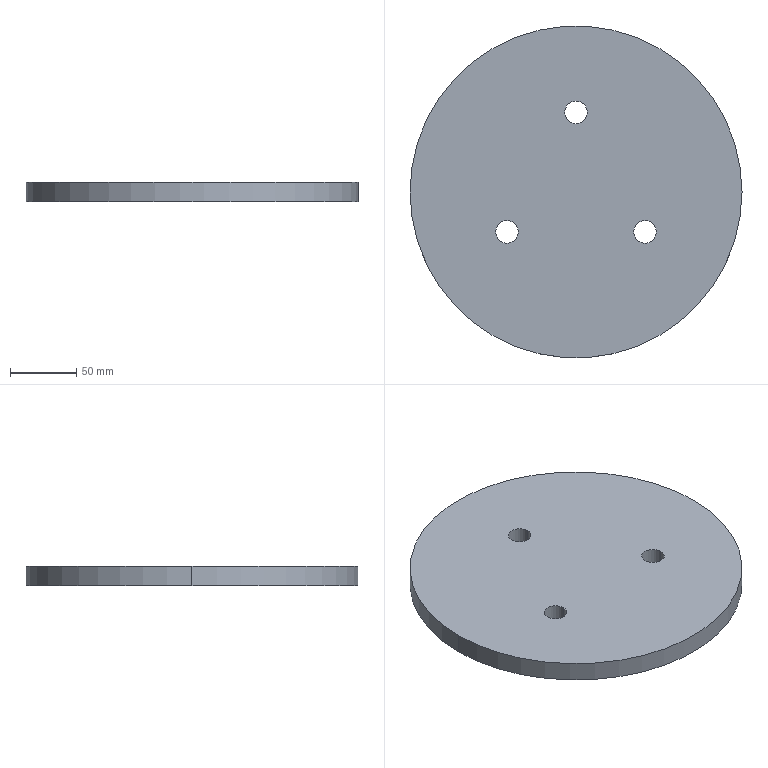Part | SolidWorks | features Extrusion 1 | 1 solid | 10 faces | box 250 x 250 x 15 mm | volume 726097 mm3 | cylinder 8 | plane 2 | commonest cylinder face diameters 17 x6 250 x2
STEP:
#1=CARTESIAN_POINT('',(-60.462,-30.,7.5));
#2=VERTEX_POINT('',#1);
#3=CARTESIAN_POINT('',(-43.462,-30.,7.5));
#4=VERTEX_POINT('',#3);
#5=CARTESIAN_POINT('',(-51.962,-30.,7.5));
#6=DIRECTION('',(0.,0.,1.));
#7=DIRECTION('',(1.,0.,0.));
#8=AXIS2_PLACEMENT_3D('',#5,#6,#7);
#9=CIRCLE('',#8,8.5);
#10=EDGE_CURVE('',#2,#4,#9,.T.);
#11=ORIENTED_EDGE('',*,*,#10,.T.);
#12=CARTESIAN_POINT('',(-43.462,-30.,-7.5));
#13=VERTEX_POINT('',#12);
#14=CARTESIAN_POINT('',(-43.462,-30.,7.5));
#15=DIRECTION('',(0.,0.,-1.));
#16=VECTOR('',#15,1000.);
#17=LINE('',#14,#16);
#18=EDGE_CURVE('',#4,#13,#17,.T.);
#19=ORIENTED_EDGE('',*,*,#18,.T.);
#20=CARTESIAN_POINT('',(-60.462,-30.,-7.5));
#21=VERTEX_POINT('',#20);
#22=CARTESIAN_POINT('',(-51.962,-30.,-7.5));
#23=DIRECTION('',(0.,0.,1.));
#24=DIRECTION('',(1.,0.,0.));
#25=AXIS2_PLACEMENT_3D('',#22,#23,#24);
#26=CIRCLE('',#25,8.5);
#27=EDGE_CURVE('',#21,#13,#26,.T.);
#28=ORIENTED_EDGE('',*,*,#27,.F.);
#29=CARTESIAN_POINT('',(-60.462,-30.,7.5));
#30=DIRECTION('',(0.,0.,-1.));
#31=VECTOR('',#30,1000.);
#32=LINE('',#29,#31);
#33=EDGE_CURVE('',#2,#21,#32,.T.);
#34=ORIENTED_EDGE('',*,*,#33,.F.);
#35=EDGE_LOOP('',(#11,#19,#28,#34));
#36=FACE_OUTER_BOUND('',#35,.T.);
#37=CARTESIAN_POINT('',(-51.962,-30.,7.5));
#38=DIRECTION('',(0.,0.,-1.));
#39=DIRECTION('',(-1.,0.,0.));
#40=AXIS2_PLACEMENT_3D('',#37,#38,#39);
#41=CYLINDRICAL_SURFACE('',#40,8.5);
#42=ADVANCED_FACE('',(#36),#41,.F.);
#43=CARTESIAN_POINT('',(43.462,-30.,7.5));
#44=VERTEX_POINT('',#43);
#45=CARTESIAN_POINT('',(60.462,-30.,7.5));
#46=VERTEX_POINT('',#45);
#47=CARTESIAN_POINT('',(51.962,-30.,7.5));
#48=DIRECTION('',(0.,0.,1.));
#49=DIRECTION('',(1.,0.,0.));
#50=AXIS2_PLACEMENT_3D('',#47,#48,#49);
#51=CIRCLE('',#50,8.5);
#52=EDGE_CURVE('',#44,#46,#51,.T.);
#53=ORIENTED_EDGE('',*,*,#52,.T.);
#54=CARTESIAN_POINT('',(60.462,-30.,-7.5));
#55=VERTEX_POINT('',#54);
#56=CARTESIAN_POINT('',(60.462,-30.,7.5));
#57=DIRECTION('',(0.,0.,-1.));
#58=VECTOR('',#57,1000.);
#59=LINE('',#56,#58);
#60=EDGE_CURVE('',#46,#55,#59,.T.);
#61=ORIENTED_EDGE('',*,*,#60,.T.);
#62=CARTESIAN_POINT('',(43.462,-30.,-7.5));
#63=VERTEX_POINT('',#62);
#64=CARTESIAN_POINT('',(51.962,-30.,-7.5));
#65=DIRECTION('',(0.,0.,1.));
#66=DIRECTION('',(1.,0.,0.));
#67=AXIS2_PLACEMENT_3D('',#64,#65,#66);
#68=CIRCLE('',#67,8.5);
#69=EDGE_CURVE('',#63,#55,#68,.T.);
#70=ORIENTED_EDGE('',*,*,#69,.F.);
#71=CARTESIAN_POINT('',(43.462,-30.,7.5));
#72=DIRECTION('',(0.,0.,-1.));
#73=VECTOR('',#72,1000.);
#74=LINE('',#71,#73);
#75=EDGE_CURVE('',#44,#63,#74,.T.);
#76=ORIENTED_EDGE('',*,*,#75,.F.);
#77=EDGE_LOOP('',(#53,#61,#70,#76));
#78=FACE_OUTER_BOUND('',#77,.T.);
#79=CARTESIAN_POINT('',(51.962,-30.,7.5));
#80=DIRECTION('',(0.,0.,-1.));
#81=DIRECTION('',(-1.,0.,0.));
#82=AXIS2_PLACEMENT_3D('',#79,#80,#81);
#83=CYLINDRICAL_SURFACE('',#82,8.5);
#84=ADVANCED_FACE('',(#78),#83,.F.);
#85=CARTESIAN_POINT('',(-8.5,60.,7.5));
#86=VERTEX_POINT('',#85);
#87=CARTESIAN_POINT('',(8.5,60.,7.5));
#88=VERTEX_POINT('',#87);
#89=CARTESIAN_POINT('',(0.,60.,7.5));
#90=DIRECTION('',(0.,0.,1.));
#91=DIRECTION('',(1.,0.,0.));
#92=AXIS2_PLACEMENT_3D('',#89,#90,#91);
#93=CIRCLE('',#92,8.5);
#94=EDGE_CURVE('',#86,#88,#93,.T.);
#95=ORIENTED_EDGE('',*,*,#94,.T.);
#96=CARTESIAN_POINT('',(8.5,60.,-7.5));
#97=VERTEX_POINT('',#96);
#98=CARTESIAN_POINT('',(8.5,60.,7.5));
#99=DIRECTION('',(0.,0.,-1.));
#100=VECTOR('',#99,1000.);
#101=LINE('',#98,#100);
#102=EDGE_CURVE('',#88,#97,#101,.T.);
#103=ORIENTED_EDGE('',*,*,#102,.T.);
#104=CARTESIAN_POINT('',(-8.5,60.,-7.5));
#105=VERTEX_POINT('',#104);
#106=CARTESIAN_POINT('',(0.,60.,-7.5));
#107=DIRECTION('',(0.,0.,1.));
#108=DIRECTION('',(1.,0.,0.));
#109=AXIS2_PLACEMENT_3D('',#106,#107,#108);
#110=CIRCLE('',#109,8.5);
#111=EDGE_CURVE('',#105,#97,#110,.T.);
#112=ORIENTED_EDGE('',*,*,#111,.F.);
#113=CARTESIAN_POINT('',(-8.5,60.,7.5));
#114=DIRECTION('',(0.,0.,-1.));
#115=VECTOR('',#114,1000.);
#116=LINE('',#113,#115);
#117=EDGE_CURVE('',#86,#105,#116,.T.);
#118=ORIENTED_EDGE('',*,*,#117,.F.);
#119=EDGE_LOOP('',(#95,#103,#112,#118));
#120=FACE_OUTER_BOUND('',#119,.T.);
#121=CARTESIAN_POINT('',(0.,60.,7.5));
#122=DIRECTION('',(0.,0.,-1.));
#123=DIRECTION('',(-1.,0.,0.));
#124=AXIS2_PLACEMENT_3D('',#121,#122,#123);
#125=CYLINDRICAL_SURFACE('',#124,8.5);
#126=ADVANCED_FACE('',(#120),#125,.F.);
#127=CARTESIAN_POINT('',(125.,0.,7.5));
#128=VERTEX_POINT('',#127);
#129=CARTESIAN_POINT('',(-125.,0.,7.5));
#130=VERTEX_POINT('',#129);
#131=CARTESIAN_POINT('',(0.,0.,7.5));
#132=DIRECTION('',(0.,0.,1.));
#133=DIRECTION('',(1.,0.,0.));
#134=AXIS2_PLACEMENT_3D('',#131,#132,#133);
#135=CIRCLE('',#134,125.);
#136=EDGE_CURVE('',#128,#130,#135,.T.);
#137=ORIENTED_EDGE('',*,*,#136,.F.);
#138=CARTESIAN_POINT('',(125.,0.,-7.5));
#139=VERTEX_POINT('',#138);
#140=CARTESIAN_POINT('',(125.,0.,7.5));
#141=DIRECTION('',(0.,0.,-1.));
#142=VECTOR('',#141,1000.);
#143=LINE('',#140,#142);
#144=EDGE_CURVE('',#128,#139,#143,.T.);
#145=ORIENTED_EDGE('',*,*,#144,.T.);
#146=CARTESIAN_POINT('',(-125.,0.,-7.5));
#147=VERTEX_POINT('',#146);
#148=CARTESIAN_POINT('',(0.,0.,-7.5));
#149=DIRECTION('',(0.,0.,1.));
#150=DIRECTION('',(1.,0.,0.));
#151=AXIS2_PLACEMENT_3D('',#148,#149,#150);
#152=CIRCLE('',#151,125.);
#153=EDGE_CURVE('',#139,#147,#152,.T.);
#154=ORIENTED_EDGE('',*,*,#153,.T.);
#155=CARTESIAN_POINT('',(-125.,0.,7.5));
#156=DIRECTION('',(0.,0.,-1.));
#157=VECTOR('',#156,1000.);
#158=LINE('',#155,#157);
#159=EDGE_CURVE('',#130,#147,#158,.T.);
#160=ORIENTED_EDGE('',*,*,#159,.F.);
#161=EDGE_LOOP('',(#137,#145,#154,#160));
#162=FACE_OUTER_BOUND('',#161,.T.);
#163=CARTESIAN_POINT('',(0.,0.,7.5));
#164=DIRECTION('',(0.,0.,-1.));
#165=DIRECTION('',(-1.,0.,0.));
#166=AXIS2_PLACEMENT_3D('',#163,#164,#165);
#167=CYLINDRICAL_SURFACE('',#166,125.);
#168=ADVANCED_FACE('',(#162),#167,.T.);
#169=ORIENTED_EDGE('',*,*,#52,.F.);
#170=CARTESIAN_POINT('',(51.962,-30.,7.5));
#171=DIRECTION('',(0.,0.,1.));
#172=DIRECTION('',(1.,0.,0.));
#173=AXIS2_PLACEMENT_3D('',#170,#171,#172);
#174=CIRCLE('',#173,8.5);
#175=EDGE_CURVE('',#46,#44,#174,.T.);
#176=ORIENTED_EDGE('',*,*,#175,.F.);
#177=EDGE_LOOP('',(#169,#176));
#178=FACE_BOUND('',#177,.T.);
#179=CARTESIAN_POINT('',(0.,0.,7.5));
#180=DIRECTION('',(0.,0.,1.));
#181=DIRECTION('',(1.,0.,0.));
#182=AXIS2_PLACEMENT_3D('',#179,#180,#181);
#183=CIRCLE('',#182,125.);
#184=EDGE_CURVE('',#130,#128,#183,.T.);
#185=ORIENTED_EDGE('',*,*,#184,.T.);
#186=ORIENTED_EDGE('',*,*,#136,.T.);
#187=EDGE_LOOP('',(#185,#186));
#188=FACE_OUTER_BOUND('',#187,.T.);
#189=ORIENTED_EDGE('',*,*,#94,.F.);
#190=CARTESIAN_POINT('',(0.,60.,7.5));
#191=DIRECTION('',(0.,0.,1.));
#192=DIRECTION('',(1.,0.,0.));
#193=AXIS2_PLACEMENT_3D('',#190,#191,#192);
#194=CIRCLE('',#193,8.5);
#195=EDGE_CURVE('',#88,#86,#194,.T.);
#196=ORIENTED_EDGE('',*,*,#195,.F.);
#197=EDGE_LOOP('',(#189,#196));
#198=FACE_BOUND('',#197,.T.);
#199=ORIENTED_EDGE('',*,*,#10,.F.);
#200=CARTESIAN_POINT('',(-51.962,-30.,7.5));
#201=DIRECTION('',(0.,0.,1.));
#202=DIRECTION('',(1.,0.,0.));
#203=AXIS2_PLACEMENT_3D('',#200,#201,#202);
#204=CIRCLE('',#203,8.5);
#205=EDGE_CURVE('',#4,#2,#204,.T.);
#206=ORIENTED_EDGE('',*,*,#205,.F.);
#207=EDGE_LOOP('',(#199,#206));
#208=FACE_BOUND('',#207,.T.);
#209=CARTESIAN_POINT('',(0.,0.,7.5));
#210=DIRECTION('',(0.,0.,1.));
#211=DIRECTION('',(1.,0.,0.));
#212=AXIS2_PLACEMENT_3D('',#209,#210,#211);
#213=PLANE('',#212);
#214=ADVANCED_FACE('',(#178,#188,#198,#208),#213,.T.);
#215=CARTESIAN_POINT('',(0.,0.,-7.5));
#216=DIRECTION('',(0.,0.,1.));
#217=DIRECTION('',(1.,0.,0.));
#218=AXIS2_PLACEMENT_3D('',#215,#216,#217);
#219=CIRCLE('',#218,125.);
#220=EDGE_CURVE('',#147,#139,#219,.T.);
#221=ORIENTED_EDGE('',*,*,#220,.F.);
#222=ORIENTED_EDGE('',*,*,#153,.F.);
#223=EDGE_LOOP('',(#221,#222));
#224=FACE_OUTER_BOUND('',#223,.T.);
#225=ORIENTED_EDGE('',*,*,#111,.T.);
#226=CARTESIAN_POINT('',(0.,60.,-7.5));
#227=DIRECTION('',(0.,0.,1.));
#228=DIRECTION('',(1.,0.,0.));
#229=AXIS2_PLACEMENT_3D('',#226,#227,#228);
#230=CIRCLE('',#229,8.5);
#231=EDGE_CURVE('',#97,#105,#230,.T.);
#232=ORIENTED_EDGE('',*,*,#231,.T.);
#233=EDGE_LOOP('',(#225,#232));
#234=FACE_BOUND('',#233,.T.);
#235=ORIENTED_EDGE('',*,*,#69,.T.);
#236=CARTESIAN_POINT('',(51.962,-30.,-7.5));
#237=DIRECTION('',(0.,0.,1.));
#238=DIRECTION('',(1.,0.,0.));
#239=AXIS2_PLACEMENT_3D('',#236,#237,#238);
#240=CIRCLE('',#239,8.5);
#241=EDGE_CURVE('',#55,#63,#240,.T.);
#242=ORIENTED_EDGE('',*,*,#241,.T.);
#243=EDGE_LOOP('',(#235,#242));
#244=FACE_BOUND('',#243,.T.);
#245=ORIENTED_EDGE('',*,*,#27,.T.);
#246=CARTESIAN_POINT('',(-51.962,-30.,-7.5));
#247=DIRECTION('',(0.,0.,1.));
#248=DIRECTION('',(1.,0.,0.));
#249=AXIS2_PLACEMENT_3D('',#246,#247,#248);
#250=CIRCLE('',#249,8.5);
#251=EDGE_CURVE('',#13,#21,#250,.T.);
#252=ORIENTED_EDGE('',*,*,#251,.T.);
#253=EDGE_LOOP('',(#245,#252));
#254=FACE_BOUND('',#253,.T.);
#255=CARTESIAN_POINT('',(0.,0.,-7.5));
#256=DIRECTION('',(0.,0.,1.));
#257=DIRECTION('',(1.,0.,0.));
#258=AXIS2_PLACEMENT_3D('',#255,#256,#257);
#259=PLANE('',#258);
#260=ADVANCED_FACE('',(#224,#234,#244,#254),#259,.F.);
#261=ORIENTED_EDGE('',*,*,#144,.F.);
#262=ORIENTED_EDGE('',*,*,#184,.F.);
#263=ORIENTED_EDGE('',*,*,#159,.T.);
#264=ORIENTED_EDGE('',*,*,#220,.T.);
#265=EDGE_LOOP('',(#261,#262,#263,#264));
#266=FACE_OUTER_BOUND('',#265,.T.);
#267=CARTESIAN_POINT('',(0.,0.,7.5));
#268=DIRECTION('',(0.,0.,-1.));
#269=DIRECTION('',(-1.,0.,0.));
#270=AXIS2_PLACEMENT_3D('',#267,#268,#269);
#271=CYLINDRICAL_SURFACE('',#270,125.);
#272=ADVANCED_FACE('',(#266),#271,.T.);
#273=ORIENTED_EDGE('',*,*,#102,.F.);
#274=ORIENTED_EDGE('',*,*,#195,.T.);
#275=ORIENTED_EDGE('',*,*,#117,.T.);
#276=ORIENTED_EDGE('',*,*,#231,.F.);
#277=EDGE_LOOP('',(#273,#274,#275,#276));
#278=FACE_OUTER_BOUND('',#277,.T.);
#279=CARTESIAN_POINT('',(0.,60.,7.5));
#280=DIRECTION('',(0.,0.,-1.));
#281=DIRECTION('',(-1.,0.,0.));
#282=AXIS2_PLACEMENT_3D('',#279,#280,#281);
#283=CYLINDRICAL_SURFACE('',#282,8.5);
#284=ADVANCED_FACE('',(#278),#283,.F.);
#285=ORIENTED_EDGE('',*,*,#60,.F.);
#286=ORIENTED_EDGE('',*,*,#175,.T.);
#287=ORIENTED_EDGE('',*,*,#75,.T.);
#288=ORIENTED_EDGE('',*,*,#241,.F.);
#289=EDGE_LOOP('',(#285,#286,#287,#288));
#290=FACE_OUTER_BOUND('',#289,.T.);
#291=CARTESIAN_POINT('',(51.962,-30.,7.5));
#292=DIRECTION('',(0.,0.,-1.));
#293=DIRECTION('',(-1.,0.,0.));
#294=AXIS2_PLACEMENT_3D('',#291,#292,#293);
#295=CYLINDRICAL_SURFACE('',#294,8.5);
#296=ADVANCED_FACE('',(#290),#295,.F.);
#297=ORIENTED_EDGE('',*,*,#18,.F.);
#298=ORIENTED_EDGE('',*,*,#205,.T.);
#299=ORIENTED_EDGE('',*,*,#33,.T.);
#300=ORIENTED_EDGE('',*,*,#251,.F.);
#301=EDGE_LOOP('',(#297,#298,#299,#300));
#302=FACE_OUTER_BOUND('',#301,.T.);
#303=CARTESIAN_POINT('',(-51.962,-30.,7.5));
#304=DIRECTION('',(0.,0.,-1.));
#305=DIRECTION('',(-1.,0.,0.));
#306=AXIS2_PLACEMENT_3D('',#303,#304,#305);
#307=CYLINDRICAL_SURFACE('',#306,8.5);
#308=ADVANCED_FACE('',(#302),#307,.F.);
#309=CLOSED_SHELL('',(#42,#84,#126,#168,#214,#260,#272,#284,#296,#308));
#310=MANIFOLD_SOLID_BREP('',#309);
#311=CARTESIAN_POINT('',(0.,0.,0.));
#312=DIRECTION('',(0.,0.,1.));
#313=DIRECTION('',(1.,0.,0.));
#314=AXIS2_PLACEMENT_3D('',#311,#312,#313);
#315=(LENGTH_UNIT()NAMED_UNIT(*)SI_UNIT(.MILLI.,.METRE.));
#316=UNCERTAINTY_MEASURE_WITH_UNIT(LENGTH_MEASURE(0.00001),#315,'','');
#317=(NAMED_UNIT(*)PLANE_ANGLE_UNIT()SI_UNIT($,.RADIAN.));
#318=(NAMED_UNIT(*)SI_UNIT($,.STERADIAN.)SOLID_ANGLE_UNIT());
#319=(GEOMETRIC_REPRESENTATION_CONTEXT(3)GLOBAL_UNCERTAINTY_ASSIGNED_CONTEXT((#316))GLOBAL_UNIT_ASSIGNED_CONTEXT((#315,#317,#318))REPRESENTATION_CONTEXT('',''));
#320=ADVANCED_BREP_SHAPE_REPRESENTATION('',(#310,#314),#319);